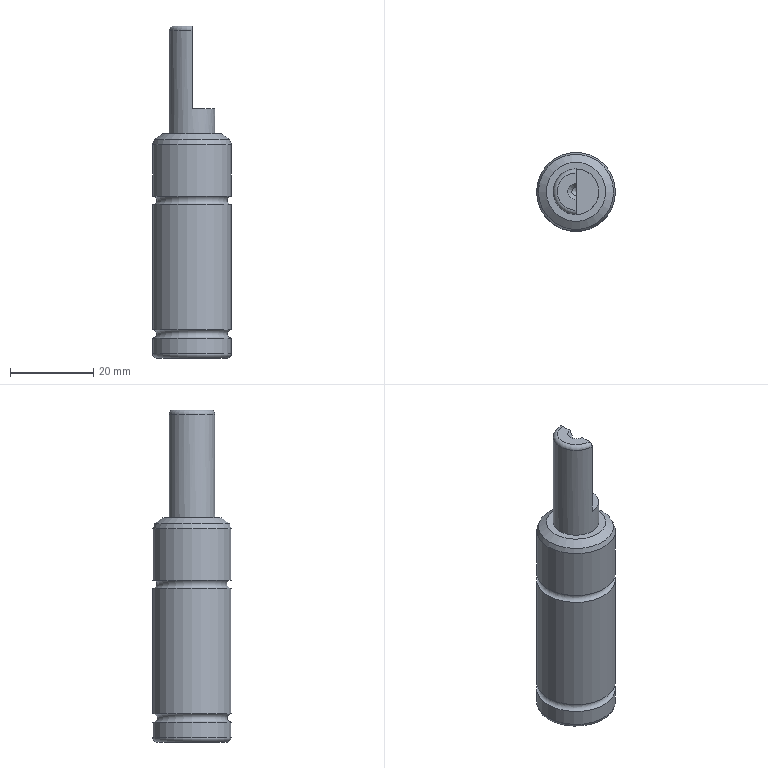Part | NX | features DG 2 | 1 solid | 152 faces | box 19 x 19 x 80 mm | volume 16395 mm3 | plane 109 | spline 29 | cylinder 6 | torus 4 | cone 4 | commonest cylinder face diameters 19 x3 2 x1 4.9 x1 11 x1